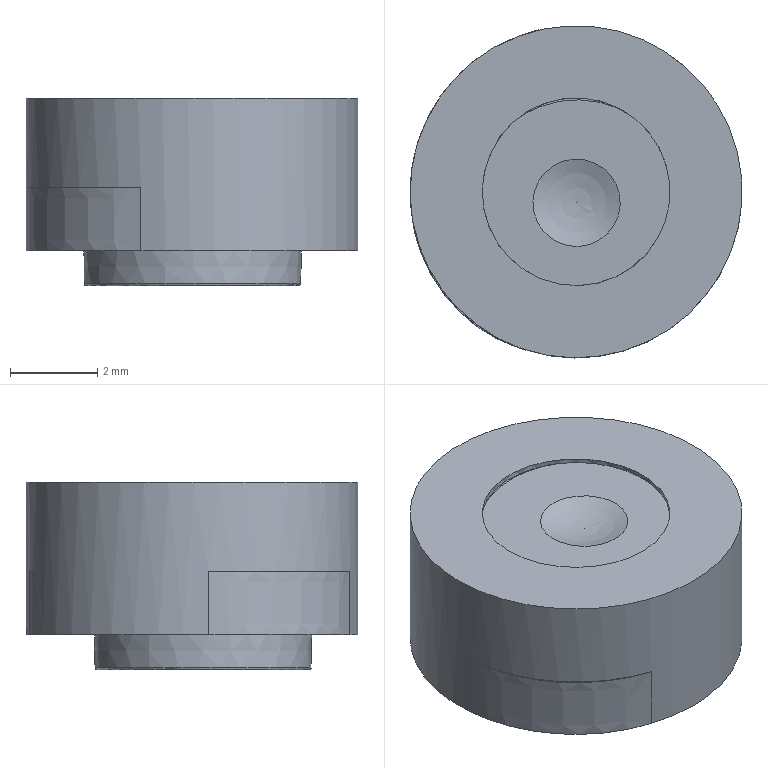Part | STEP file | 1 solid | 29 faces | box 7.6 x 7.6 x 4.3 mm | volume 142.649 mm3 | plane 14 | cylinder 9 | torus 2 | sphere 2 | other 1 | cone 1 | commonest cylinder face diameters 0.1 x6 4.3 x1 7.6 x1 8.471 x1
STEP:
#1=CARTESIAN_POINT('',(24.063,11.212,-13.81));
#2=VERTEX_POINT('',#1);
#3=CARTESIAN_POINT('',(21.454,14.437,-13.81));
#4=VERTEX_POINT('',#3);
#5=CARTESIAN_POINT('',(25.234,14.827,-13.81));
#6=DIRECTION('',(0.,0.,-1.));
#7=DIRECTION('',(-0.3082,-0.9513,0.));
#8=AXIS2_PLACEMENT_3D('',#5,#6,#7);
#9=CIRCLE('',#8,3.8);
#10=EDGE_CURVE('',#2,#4,#9,.T.);
#11=ORIENTED_EDGE('',*,*,#10,.T.);
#12=CARTESIAN_POINT('',(21.454,14.437,-13.81));
#13=CARTESIAN_POINT('',(21.456,14.416,-13.81));
#14=CARTESIAN_POINT('',(21.46,14.376,-13.81));
#15=CARTESIAN_POINT('',(21.467,14.316,-13.81));
#16=CARTESIAN_POINT('',(21.474,14.255,-13.81));
#17=CARTESIAN_POINT('',(21.48,14.215,-13.81));
#18=CARTESIAN_POINT('',(21.486,14.175,-13.81));
#19=CARTESIAN_POINT('',(21.493,14.135,-13.81));
#20=CARTESIAN_POINT('',(21.503,14.076,-13.81));
#21=CARTESIAN_POINT('',(21.515,14.017,-13.81));
#22=CARTESIAN_POINT('',(21.527,13.958,-13.81));
#23=CARTESIAN_POINT('',(21.54,13.899,-13.81));
#24=CARTESIAN_POINT('',(21.554,13.841,-13.81));
#25=CARTESIAN_POINT('',(21.569,13.783,-13.81));
#26=CARTESIAN_POINT('',(21.58,13.745,-13.81));
#27=CARTESIAN_POINT('',(21.591,13.706,-13.81));
#28=CARTESIAN_POINT('',(21.603,13.667,-13.81));
#29=CARTESIAN_POINT('',(21.62,13.61,-13.81));
#30=CARTESIAN_POINT('',(21.639,13.554,-13.81));
#31=CARTESIAN_POINT('',(21.659,13.498,-13.81));
#32=CARTESIAN_POINT('',(21.679,13.441,-13.81));
#33=CARTESIAN_POINT('',(21.701,13.384,-13.81));
#34=CARTESIAN_POINT('',(21.723,13.331,-13.81));
#35=CARTESIAN_POINT('',(21.74,13.291,-13.81));
#36=CARTESIAN_POINT('',(21.758,13.248,-13.81));
#37=CARTESIAN_POINT('',(21.782,13.194,-13.81));
#38=CARTESIAN_POINT('',(21.816,13.123,-13.81));
#39=CARTESIAN_POINT('',(21.842,13.07,-13.81));
#40=CARTESIAN_POINT('',(21.878,13.001,-13.81));
#41=CARTESIAN_POINT('',(21.919,12.925,-13.81));
#42=CARTESIAN_POINT('',(21.966,12.844,-13.81));
#43=CARTESIAN_POINT('',(22.015,12.764,-13.81));
#44=CARTESIAN_POINT('',(22.065,12.686,-13.81));
#45=CARTESIAN_POINT('',(22.127,12.597,-13.81));
#46=CARTESIAN_POINT('',(22.179,12.526,-13.81));
#47=CARTESIAN_POINT('',(22.217,12.476,-13.81));
#48=CARTESIAN_POINT('',(22.249,12.434,-13.81));
#49=CARTESIAN_POINT('',(22.285,12.391,-13.81));
#50=CARTESIAN_POINT('',(22.337,12.328,-13.81));
#51=CARTESIAN_POINT('',(22.409,12.247,-13.81));
#52=CARTESIAN_POINT('',(22.48,12.171,-13.81));
#53=CARTESIAN_POINT('',(22.546,12.105,-13.81));
#54=CARTESIAN_POINT('',(22.613,12.041,-13.81));
#55=CARTESIAN_POINT('',(22.686,11.974,-13.81));
#56=CARTESIAN_POINT('',(22.765,11.906,-13.81));
#57=CARTESIAN_POINT('',(22.828,11.854,-13.81));
#58=CARTESIAN_POINT('',(22.871,11.821,-13.81));
#59=CARTESIAN_POINT('',(22.907,11.794,-13.81));
#60=CARTESIAN_POINT('',(22.942,11.767,-13.81));
#61=CARTESIAN_POINT('',(22.991,11.732,-13.81));
#62=CARTESIAN_POINT('',(23.041,11.697,-13.81));
#63=CARTESIAN_POINT('',(23.091,11.663,-13.81));
#64=CARTESIAN_POINT('',(23.142,11.63,-13.81));
#65=CARTESIAN_POINT('',(23.194,11.597,-13.81));
#66=CARTESIAN_POINT('',(23.235,11.573,-13.81));
#67=CARTESIAN_POINT('',(23.271,11.552,-13.81));
#68=CARTESIAN_POINT('',(23.308,11.531,-13.81));
#69=CARTESIAN_POINT('',(23.361,11.501,-13.81));
#70=CARTESIAN_POINT('',(23.426,11.466,-13.81));
#71=CARTESIAN_POINT('',(23.509,11.425,-13.81));
#72=CARTESIAN_POINT('',(23.579,11.392,-13.81));
#73=CARTESIAN_POINT('',(23.654,11.359,-13.81));
#74=CARTESIAN_POINT('',(23.73,11.327,-13.81));
#75=CARTESIAN_POINT('',(23.832,11.288,-13.81));
#76=CARTESIAN_POINT('',(23.906,11.262,-13.81));
#77=CARTESIAN_POINT('',(23.981,11.237,-13.81));
#78=CARTESIAN_POINT('',(24.022,11.224,-13.81));
#79=CARTESIAN_POINT('',(24.063,11.212,-13.81));
#80=B_SPLINE_CURVE_WITH_KNOTS('',3,(#12,#13,#14,#15,#16,#17,#18,#19,#20,#21,#22,#23,#24,#25,#26,#27,#28,#29,#30,#31,#32,#33,#34,#35,#36,#37,#38,#39,#40,#41,#42,#43,#44,#45,#46,#47,#48,#49,#50,#51,#52,#53,#54,#55,#56,#57,#58,#59,#60,#61,#62,#63,#64,#65,#66,#67,#68,#69,#70,#71,#72,#73,#74,#75,#76,#77,#78,#79),.UNSPECIFIED.,.F.,.F.,(4,1,1,1,1,1,1,1,1,1,1,1,1,1,1,1,1,1,1,1,1,1,1,1,1,1,1,1,1,1,1,1,1,1,1,1,1,1,1,1,1,1,1,1,1,1,1,1,1,1,1,1,1,1,1,1,1,1,1,1,1,1,1,1,1,4),(0.,0.01381,0.02762,0.04141,0.05518,0.05537,0.06892,0.08262,0.0963,0.1099,0.1236,0.1372,0.1509,0.164,0.1645,0.1781,0.1916,0.2052,0.2187,0.2321,0.2461,0.2606,0.2707,0.276,0.292,0.311,0.3293,0.3324,0.3643,0.3876,0.3963,0.4283,0.4504,0.4704,0.4885,0.4928,0.5065,0.5266,0.5485,0.5803,0.5972,0.612,0.6435,0.6646,0.6832,0.6989,0.7013,0.7141,0.7285,0.7425,0.756,0.7697,0.7836,0.7978,0.8019,0.8123,0.8269,0.8435,0.8621,0.8898,0.8961,0.9178,0.946,0.971,0.9711,1.),.UNSPECIFIED.);
#81=EDGE_CURVE('',#4,#2,#80,.T.);
#82=ORIENTED_EDGE('',*,*,#81,.T.);
#83=EDGE_LOOP('',(#11,#82));
#84=FACE_BOUND('',#83,.T.);
#85=CARTESIAN_POINT('',(25.245,14.575,-13.81));
#86=DIRECTION('',(0.,0.,1.));
#87=DIRECTION('',(1.,0.,0.));
#88=AXIS2_PLACEMENT_3D('',#85,#86,#87);
#89=PLANE('',#88);
#90=ADVANCED_FACE('',(#84),#89,.T.);
#91=ORIENTED_EDGE('',*,*,#81,.F.);
#92=CARTESIAN_POINT('',(21.454,14.437,-15.26));
#93=VERTEX_POINT('',#92);
#94=CARTESIAN_POINT('',(21.454,14.437,-13.81));
#95=DIRECTION('',(0.,0.,-1.));
#96=VECTOR('',#95,1.);
#97=LINE('',#94,#96);
#98=EDGE_CURVE('',#4,#93,#97,.T.);
#99=ORIENTED_EDGE('',*,*,#98,.T.);
#100=CARTESIAN_POINT('',(24.063,11.212,-15.26));
#101=VERTEX_POINT('',#100);
#102=CARTESIAN_POINT('',(24.063,11.212,-15.26));
#103=CARTESIAN_POINT('',(24.014,11.226,-15.26));
#104=CARTESIAN_POINT('',(23.942,11.249,-15.26));
#105=CARTESIAN_POINT('',(23.846,11.283,-15.26));
#106=CARTESIAN_POINT('',(23.752,11.318,-15.26));
#107=CARTESIAN_POINT('',(23.635,11.366,-15.26));
#108=CARTESIAN_POINT('',(23.52,11.419,-15.26));
#109=CARTESIAN_POINT('',(23.43,11.465,-15.26));
#110=CARTESIAN_POINT('',(23.34,11.512,-15.26));
#111=CARTESIAN_POINT('',(23.229,11.576,-15.26));
#112=CARTESIAN_POINT('',(23.123,11.642,-15.26));
#113=CARTESIAN_POINT('',(23.038,11.699,-15.26));
#114=CARTESIAN_POINT('',(22.955,11.757,-15.26));
#115=CARTESIAN_POINT('',(22.889,11.807,-15.26));
#116=CARTESIAN_POINT('',(22.809,11.87,-15.26));
#117=CARTESIAN_POINT('',(22.742,11.925,-15.26));
#118=CARTESIAN_POINT('',(22.67,11.988,-15.26));
#119=CARTESIAN_POINT('',(22.6,12.052,-15.26));
#120=CARTESIAN_POINT('',(22.526,12.124,-15.26));
#121=CARTESIAN_POINT('',(22.434,12.219,-15.26));
#122=CARTESIAN_POINT('',(22.37,12.29,-15.26));
#123=CARTESIAN_POINT('',(22.316,12.353,-15.26));
#124=CARTESIAN_POINT('',(22.265,12.414,-15.26));
#125=CARTESIAN_POINT('',(22.196,12.502,-15.26));
#126=CARTESIAN_POINT('',(22.125,12.6,-15.26));
#127=CARTESIAN_POINT('',(22.078,12.668,-15.26));
#128=CARTESIAN_POINT('',(22.027,12.745,-15.26));
#129=CARTESIAN_POINT('',(21.964,12.846,-15.26));
#130=CARTESIAN_POINT('',(21.888,12.98,-15.26));
#131=CARTESIAN_POINT('',(21.824,13.105,-15.26));
#132=CARTESIAN_POINT('',(21.765,13.231,-15.26));
#133=CARTESIAN_POINT('',(21.706,13.369,-15.26));
#134=CARTESIAN_POINT('',(21.663,13.484,-15.26));
#135=CARTESIAN_POINT('',(21.634,13.568,-15.26));
#136=CARTESIAN_POINT('',(21.61,13.642,-15.26));
#137=CARTESIAN_POINT('',(21.579,13.745,-15.26));
#138=CARTESIAN_POINT('',(21.553,13.846,-15.26));
#139=CARTESIAN_POINT('',(21.534,13.928,-15.26));
#140=CARTESIAN_POINT('',(21.52,13.99,-15.26));
#141=CARTESIAN_POINT('',(21.508,14.049,-15.26));
#142=CARTESIAN_POINT('',(21.495,14.121,-15.26));
#143=CARTESIAN_POINT('',(21.482,14.204,-15.26));
#144=CARTESIAN_POINT('',(21.472,14.273,-15.26));
#145=CARTESIAN_POINT('',(21.466,14.325,-15.26));
#146=CARTESIAN_POINT('',(21.46,14.376,-15.26));
#147=CARTESIAN_POINT('',(21.457,14.412,-15.26));
#148=CARTESIAN_POINT('',(21.454,14.437,-15.26));
#149=B_SPLINE_CURVE_WITH_KNOTS('',3,(#102,#103,#104,#105,#106,#107,#108,#109,#110,#111,#112,#113,#114,#115,#116,#117,#118,#119,#120,#121,#122,#123,#124,#125,#126,#127,#128,#129,#130,#131,#132,#133,#134,#135,#136,#137,#138,#139,#140,#141,#142,#143,#144,#145,#146,#147,#148),.UNSPECIFIED.,.F.,.F.,(4,1,1,1,1,1,1,1,1,1,1,1,1,1,1,1,1,1,1,1,1,1,1,1,1,1,1,1,1,1,1,1,1,1,1,1,1,1,1,1,1,1,1,1,4),(0.,0.03441,0.05187,0.06883,0.1032,0.1378,0.1548,0.1723,0.207,0.2417,0.257,0.2766,0.3114,0.3132,0.3454,0.3704,0.3786,0.4099,0.4404,0.469,0.4746,0.4968,0.5236,0.5503,0.5794,0.5801,0.6129,0.6604,0.6852,0.708,0.7555,0.7875,0.7914,0.8161,0.8405,0.8644,0.8868,0.8977,0.9081,0.9279,0.9471,0.9653,0.9755,0.9829,1.),.UNSPECIFIED.);
#150=EDGE_CURVE('',#101,#93,#149,.T.);
#151=ORIENTED_EDGE('',*,*,#150,.F.);
#152=CARTESIAN_POINT('',(24.063,11.212,-15.26));
#153=DIRECTION('',(0.,0.,1.));
#154=VECTOR('',#153,1.);
#155=LINE('',#152,#154);
#156=EDGE_CURVE('',#101,#2,#155,.T.);
#157=ORIENTED_EDGE('',*,*,#156,.T.);
#158=EDGE_LOOP('',(#91,#99,#151,#157));
#159=FACE_BOUND('',#158,.T.);
#160=CARTESIAN_POINT('',(24.179,11.181,-13.781));
#161=CARTESIAN_POINT('',(24.14,11.19,-13.781));
#162=CARTESIAN_POINT('',(23.887,11.26,-13.781));
#163=CARTESIAN_POINT('',(23.197,11.533,-13.781));
#164=CARTESIAN_POINT('',(22.25,12.283,-13.781));
#165=CARTESIAN_POINT('',(21.632,13.394,-13.781));
#166=CARTESIAN_POINT('',(21.471,14.194,-13.781));
#167=CARTESIAN_POINT('',(21.448,14.516,-13.781));
#168=CARTESIAN_POINT('',(21.446,14.556,-13.781));
#169=B_SPLINE_CURVE_WITH_KNOTS('',3,(#160,#161,#162,#163,#164,#165,#166,#167,#168),.UNSPECIFIED.,.F.,.F.,(4,1,1,1,1,1,4),(0.,0.02582,0.1691,0.477,0.7911,0.9742,1.),.UNSPECIFIED.);
#170=DIRECTION('',(0.,0.,-1.));
#171=VECTOR('',#170,1.);
#172=SURFACE_OF_LINEAR_EXTRUSION('',#169,#171);
#173=ADVANCED_FACE('',(#159),#172,.T.);
#174=CARTESIAN_POINT('',(28.525,12.927,-11.76));
#175=VERTEX_POINT('',#174);
#176=CARTESIAN_POINT('',(25.234,14.827,-11.76));
#177=DIRECTION('',(0.,0.,1.));
#178=DIRECTION('',(-0.866,0.5,0.));
#179=AXIS2_PLACEMENT_3D('',#176,#177,#178);
#180=CIRCLE('',#179,3.8);
#181=EDGE_CURVE('',#175,#175,#180,.T.);
#182=ORIENTED_EDGE('',*,*,#181,.F.);
#183=EDGE_LOOP('',(#182));
#184=FACE_OUTER_BOUND('',#183,.T.);
#185=CARTESIAN_POINT('',(24.39,18.532,-15.26));
#186=VERTEX_POINT('',#185);
#187=CARTESIAN_POINT('',(28.525,12.927,-15.26));
#188=VERTEX_POINT('',#187);
#189=CARTESIAN_POINT('',(25.234,14.827,-15.26));
#190=DIRECTION('',(0.,0.,-1.));
#191=DIRECTION('',(-0.2221,0.975,0.));
#192=AXIS2_PLACEMENT_3D('',#189,#190,#191);
#193=CIRCLE('',#192,3.8);
#194=EDGE_CURVE('',#186,#188,#193,.T.);
#195=ORIENTED_EDGE('',*,*,#194,.F.);
#196=CARTESIAN_POINT('',(24.39,18.532,-13.81));
#197=VERTEX_POINT('',#196);
#198=CARTESIAN_POINT('',(24.39,18.532,-15.26));
#199=DIRECTION('',(0.,0.,1.));
#200=VECTOR('',#199,1.);
#201=LINE('',#198,#200);
#202=EDGE_CURVE('',#186,#197,#201,.T.);
#203=ORIENTED_EDGE('',*,*,#202,.T.);
#204=CARTESIAN_POINT('',(24.092,18.451,-13.81));
#205=VERTEX_POINT('',#204);
#206=CARTESIAN_POINT('',(25.234,14.827,-13.81));
#207=DIRECTION('',(0.,0.,-1.));
#208=DIRECTION('',(-0.3006,0.9537,0.));
#209=AXIS2_PLACEMENT_3D('',#206,#207,#208);
#210=CIRCLE('',#209,3.8);
#211=EDGE_CURVE('',#205,#197,#210,.T.);
#212=ORIENTED_EDGE('',*,*,#211,.F.);
#213=CARTESIAN_POINT('',(24.092,18.451,-15.26));
#214=VERTEX_POINT('',#213);
#215=CARTESIAN_POINT('',(24.092,18.451,-15.26));
#216=DIRECTION('',(0.,0.,1.));
#217=VECTOR('',#216,1.);
#218=LINE('',#215,#217);
#219=EDGE_CURVE('',#214,#205,#218,.T.);
#220=ORIENTED_EDGE('',*,*,#219,.F.);
#221=CARTESIAN_POINT('',(25.234,14.827,-15.26));
#222=DIRECTION('',(0.,0.,-1.));
#223=DIRECTION('',(-0.9947,-0.1028,0.));
#224=AXIS2_PLACEMENT_3D('',#221,#222,#223);
#225=CIRCLE('',#224,3.8);
#226=EDGE_CURVE('',#93,#214,#225,.T.);
#227=ORIENTED_EDGE('',*,*,#226,.F.);
#228=ORIENTED_EDGE('',*,*,#98,.F.);
#229=ORIENTED_EDGE('',*,*,#10,.F.);
#230=ORIENTED_EDGE('',*,*,#156,.F.);
#231=CARTESIAN_POINT('',(25.234,14.827,-15.26));
#232=DIRECTION('',(0.,0.,-1.));
#233=DIRECTION('',(0.866,-0.5,0.));
#234=AXIS2_PLACEMENT_3D('',#231,#232,#233);
#235=CIRCLE('',#234,3.8);
#236=EDGE_CURVE('',#188,#101,#235,.T.);
#237=ORIENTED_EDGE('',*,*,#236,.F.);
#238=EDGE_LOOP('',(#195,#203,#212,#220,#227,#228,#229,#230,#237));
#239=FACE_BOUND('',#238,.T.);
#240=CARTESIAN_POINT('',(25.234,14.827,-15.26));
#241=DIRECTION('',(0.,0.,1.));
#242=DIRECTION('',(0.866,-0.5,0.));
#243=AXIS2_PLACEMENT_3D('',#240,#241,#242);
#244=CYLINDRICAL_SURFACE('',#243,3.8);
#245=ADVANCED_FACE('',(#184,#239),#244,.T.);
#246=ORIENTED_EDGE('',*,*,#194,.T.);
#247=ORIENTED_EDGE('',*,*,#236,.T.);
#248=ORIENTED_EDGE('',*,*,#150,.T.);
#249=ORIENTED_EDGE('',*,*,#226,.T.);
#250=CARTESIAN_POINT('',(24.375,18.541,-15.26));
#251=VERTEX_POINT('',#250);
#252=CARTESIAN_POINT('',(25.507,14.459,-15.26));
#253=DIRECTION('',(0.,0.,-1.));
#254=DIRECTION('',(-0.3341,0.9425,0.));
#255=AXIS2_PLACEMENT_3D('',#252,#253,#254);
#256=CIRCLE('',#255,4.236);
#257=EDGE_CURVE('',#214,#251,#256,.T.);
#258=ORIENTED_EDGE('',*,*,#257,.T.);
#259=CARTESIAN_POINT('',(24.375,18.541,-15.26));
#260=DIRECTION('',(0.866,-0.5,0.));
#261=VECTOR('',#260,1.);
#262=LINE('',#259,#261);
#263=EDGE_CURVE('',#251,#186,#262,.T.);
#264=ORIENTED_EDGE('',*,*,#263,.T.);
#265=EDGE_LOOP('',(#246,#247,#248,#249,#258,#264));
#266=FACE_BOUND('',#265,.T.);
#267=CARTESIAN_POINT('',(23.088,15.82,-15.26));
#268=VERTEX_POINT('',#267);
#269=CARTESIAN_POINT('',(25.245,14.575,-15.26));
#270=DIRECTION('',(0.,0.,1.));
#271=DIRECTION('',(1.,0.,0.));
#272=AXIS2_PLACEMENT_3D('',#269,#270,#271);
#273=CIRCLE('',#272,2.49);
#274=EDGE_CURVE('',#268,#268,#273,.T.);
#275=ORIENTED_EDGE('',*,*,#274,.T.);
#276=EDGE_LOOP('',(#275));
#277=FACE_BOUND('',#276,.T.);
#278=CARTESIAN_POINT('',(25.245,14.575,-15.26));
#279=DIRECTION('',(0.,0.,1.));
#280=DIRECTION('',(1.,0.,0.));
#281=AXIS2_PLACEMENT_3D('',#278,#279,#280);
#282=PLANE('',#281);
#283=ADVANCED_FACE('',(#266,#277),#282,.F.);
#284=CARTESIAN_POINT('',(24.375,18.541,-13.81));
#285=VERTEX_POINT('',#284);
#286=CARTESIAN_POINT('',(24.39,18.532,-13.81));
#287=DIRECTION('',(-0.866,0.5,0.));
#288=VECTOR('',#287,1.);
#289=LINE('',#286,#288);
#290=EDGE_CURVE('',#197,#285,#289,.T.);
#291=ORIENTED_EDGE('',*,*,#290,.F.);
#292=ORIENTED_EDGE('',*,*,#202,.F.);
#293=ORIENTED_EDGE('',*,*,#263,.F.);
#294=CARTESIAN_POINT('',(24.375,18.541,-13.81));
#295=DIRECTION('',(0.,0.,-1.));
#296=VECTOR('',#295,1.);
#297=LINE('',#294,#296);
#298=EDGE_CURVE('',#285,#251,#297,.T.);
#299=ORIENTED_EDGE('',*,*,#298,.F.);
#300=EDGE_LOOP('',(#291,#292,#293,#299));
#301=FACE_BOUND('',#300,.T.);
#302=CARTESIAN_POINT('',(26.745,17.173,-15.26));
#303=DIRECTION('',(-0.5,-0.866,0.));
#304=DIRECTION('',(-0.866,0.5,0.));
#305=AXIS2_PLACEMENT_3D('',#302,#303,#304);
#306=PLANE('',#305);
#307=ADVANCED_FACE('',(#301),#306,.F.);
#308=CARTESIAN_POINT('',(25.507,14.459,-13.81));
#309=DIRECTION('',(0.,0.,1.));
#310=DIRECTION('',(-0.2671,0.9637,0.));
#311=AXIS2_PLACEMENT_3D('',#308,#309,#310);
#312=CIRCLE('',#311,4.236);
#313=EDGE_CURVE('',#285,#205,#312,.T.);
#314=ORIENTED_EDGE('',*,*,#313,.F.);
#315=ORIENTED_EDGE('',*,*,#298,.T.);
#316=ORIENTED_EDGE('',*,*,#257,.F.);
#317=ORIENTED_EDGE('',*,*,#219,.T.);
#318=EDGE_LOOP('',(#314,#315,#316,#317));
#319=FACE_BOUND('',#318,.T.);
#320=CARTESIAN_POINT('',(25.507,14.459,-14.535));
#321=DIRECTION('',(0.,0.,1.));
#322=DIRECTION('',(-0.3341,0.9425,0.));
#323=AXIS2_PLACEMENT_3D('',#320,#321,#322);
#324=CYLINDRICAL_SURFACE('',#323,4.236);
#325=ADVANCED_FACE('',(#319),#324,.T.);
#326=ORIENTED_EDGE('',*,*,#313,.T.);
#327=ORIENTED_EDGE('',*,*,#211,.T.);
#328=ORIENTED_EDGE('',*,*,#290,.T.);
#329=EDGE_LOOP('',(#326,#327,#328));
#330=FACE_BOUND('',#329,.T.);
#331=CARTESIAN_POINT('',(25.245,14.575,-13.81));
#332=DIRECTION('',(0.,0.,1.));
#333=DIRECTION('',(1.,0.,0.));
#334=AXIS2_PLACEMENT_3D('',#331,#332,#333);
#335=PLANE('',#334);
#336=ADVANCED_FACE('',(#330),#335,.T.);
#337=CARTESIAN_POINT('',(23.1,15.813,-16.011));
#338=VERTEX_POINT('',#337);
#339=CARTESIAN_POINT('',(23.1,15.813,-16.011));
#340=CARTESIAN_POINT('',(23.126,15.858,-16.011));
#341=CARTESIAN_POINT('',(23.18,15.947,-16.011));
#342=CARTESIAN_POINT('',(23.27,16.074,-16.011));
#343=CARTESIAN_POINT('',(23.368,16.195,-16.011));
#344=CARTESIAN_POINT('',(23.474,16.309,-16.011));
#345=CARTESIAN_POINT('',(23.586,16.417,-16.011));
#346=CARTESIAN_POINT('',(23.705,16.517,-16.011));
#347=CARTESIAN_POINT('',(23.83,16.61,-16.011));
#348=CARTESIAN_POINT('',(23.961,16.695,-16.011));
#349=CARTESIAN_POINT('',(24.097,16.772,-16.011));
#350=CARTESIAN_POINT('',(24.237,16.839,-16.011));
#351=CARTESIAN_POINT('',(24.381,16.898,-16.011));
#352=CARTESIAN_POINT('',(24.529,16.948,-16.011));
#353=CARTESIAN_POINT('',(24.679,16.988,-16.011));
#354=CARTESIAN_POINT('',(24.832,17.019,-16.011));
#355=CARTESIAN_POINT('',(24.986,17.04,-16.011));
#356=CARTESIAN_POINT('',(25.141,17.051,-16.011));
#357=CARTESIAN_POINT('',(25.297,17.053,-16.011));
#358=CARTESIAN_POINT('',(25.452,17.045,-16.011));
#359=CARTESIAN_POINT('',(25.607,17.027,-16.011));
#360=CARTESIAN_POINT('',(25.76,16.999,-16.011));
#361=CARTESIAN_POINT('',(25.912,16.962,-16.011));
#362=CARTESIAN_POINT('',(26.06,16.915,-16.011));
#363=CARTESIAN_POINT('',(26.206,16.86,-16.011));
#364=CARTESIAN_POINT('',(26.347,16.795,-16.011));
#365=CARTESIAN_POINT('',(26.484,16.721,-16.011));
#366=CARTESIAN_POINT('',(26.617,16.639,-16.011));
#367=CARTESIAN_POINT('',(26.744,16.549,-16.011));
#368=CARTESIAN_POINT('',(26.865,16.451,-16.011));
#369=CARTESIAN_POINT('',(26.979,16.345,-16.011));
#370=CARTESIAN_POINT('',(27.087,16.233,-16.011));
#371=CARTESIAN_POINT('',(27.188,16.114,-16.011));
#372=CARTESIAN_POINT('',(27.28,15.989,-16.011));
#373=CARTESIAN_POINT('',(27.365,15.858,-16.011));
#374=CARTESIAN_POINT('',(27.442,15.723,-16.011));
#375=CARTESIAN_POINT('',(27.509,15.582,-16.011));
#376=CARTESIAN_POINT('',(27.568,15.438,-16.011));
#377=CARTESIAN_POINT('',(27.618,15.29,-16.011));
#378=CARTESIAN_POINT('',(27.658,15.14,-16.011));
#379=CARTESIAN_POINT('',(27.689,14.987,-16.011));
#380=CARTESIAN_POINT('',(27.71,14.833,-16.011));
#381=CARTESIAN_POINT('',(27.721,14.678,-16.011));
#382=CARTESIAN_POINT('',(27.723,14.522,-16.011));
#383=CARTESIAN_POINT('',(27.714,14.367,-16.011));
#384=CARTESIAN_POINT('',(27.696,14.212,-16.011));
#385=CARTESIAN_POINT('',(27.669,14.059,-16.011));
#386=CARTESIAN_POINT('',(27.632,13.907,-16.011));
#387=CARTESIAN_POINT('',(27.585,13.759,-16.011));
#388=CARTESIAN_POINT('',(27.529,13.613,-16.011));
#389=CARTESIAN_POINT('',(27.464,13.472,-16.011));
#390=CARTESIAN_POINT('',(27.415,13.381,-16.011));
#391=CARTESIAN_POINT('',(27.39,13.337,-16.011));
#392=CARTESIAN_POINT('',(27.364,13.292,-16.011));
#393=CARTESIAN_POINT('',(27.309,13.203,-16.011));
#394=CARTESIAN_POINT('',(27.219,13.076,-16.011));
#395=CARTESIAN_POINT('',(27.121,12.955,-16.011));
#396=CARTESIAN_POINT('',(27.015,12.841,-16.011));
#397=CARTESIAN_POINT('',(26.903,12.733,-16.011));
#398=CARTESIAN_POINT('',(26.784,12.633,-16.011));
#399=CARTESIAN_POINT('',(26.659,12.54,-16.011));
#400=CARTESIAN_POINT('',(26.528,12.455,-16.011));
#401=CARTESIAN_POINT('',(26.393,12.378,-16.011));
#402=CARTESIAN_POINT('',(26.253,12.311,-16.011));
#403=CARTESIAN_POINT('',(26.108,12.252,-16.011));
#404=CARTESIAN_POINT('',(25.961,12.202,-16.011));
#405=CARTESIAN_POINT('',(25.81,12.162,-16.011));
#406=CARTESIAN_POINT('',(25.658,12.131,-16.011));
#407=CARTESIAN_POINT('',(25.503,12.11,-16.011));
#408=CARTESIAN_POINT('',(25.348,12.099,-16.011));
#409=CARTESIAN_POINT('',(25.192,12.097,-16.011));
#410=CARTESIAN_POINT('',(25.037,12.105,-16.011));
#411=CARTESIAN_POINT('',(24.882,12.123,-16.011));
#412=CARTESIAN_POINT('',(24.729,12.151,-16.011));
#413=CARTESIAN_POINT('',(24.578,12.188,-16.011));
#414=CARTESIAN_POINT('',(24.429,12.235,-16.011));
#415=CARTESIAN_POINT('',(24.284,12.29,-16.011));
#416=CARTESIAN_POINT('',(24.142,12.355,-16.011));
#417=CARTESIAN_POINT('',(24.005,12.429,-16.011));
#418=CARTESIAN_POINT('',(23.873,12.511,-16.011));
#419=CARTESIAN_POINT('',(23.746,12.601,-16.011));
#420=CARTESIAN_POINT('',(23.625,12.699,-16.011));
#421=CARTESIAN_POINT('',(23.51,12.805,-16.011));
#422=CARTESIAN_POINT('',(23.402,12.917,-16.011));
#423=CARTESIAN_POINT('',(23.302,13.036,-16.011));
#424=CARTESIAN_POINT('',(23.209,13.161,-16.011));
#425=CARTESIAN_POINT('',(23.124,13.292,-16.011));
#426=CARTESIAN_POINT('',(23.048,13.427,-16.011));
#427=CARTESIAN_POINT('',(22.98,13.568,-16.011));
#428=CARTESIAN_POINT('',(22.921,13.712,-16.011));
#429=CARTESIAN_POINT('',(22.872,13.86,-16.011));
#430=CARTESIAN_POINT('',(22.831,14.01,-16.011));
#431=CARTESIAN_POINT('',(22.801,14.163,-16.011));
#432=CARTESIAN_POINT('',(22.78,14.317,-16.011));
#433=CARTESIAN_POINT('',(22.768,14.472,-16.011));
#434=CARTESIAN_POINT('',(22.767,14.628,-16.011));
#435=CARTESIAN_POINT('',(22.775,14.783,-16.011));
#436=CARTESIAN_POINT('',(22.793,14.938,-16.011));
#437=CARTESIAN_POINT('',(22.821,15.091,-16.011));
#438=CARTESIAN_POINT('',(22.858,15.243,-16.011));
#439=CARTESIAN_POINT('',(22.904,15.391,-16.011));
#440=CARTESIAN_POINT('',(22.96,15.537,-16.011));
#441=CARTESIAN_POINT('',(23.025,15.678,-16.011));
#442=CARTESIAN_POINT('',(23.074,15.769,-16.011));
#443=CARTESIAN_POINT('',(23.1,15.813,-16.011));
#444=B_SPLINE_CURVE_WITH_KNOTS('',3,(#339,#340,#341,#342,#343,#344,#345,#346,#347,#348,#349,#350,#351,#352,#353,#354,#355,#356,#357,#358,#359,#360,#361,#362,#363,#364,#365,#366,#367,#368,#369,#370,#371,#372,#373,#374,#375,#376,#377,#378,#379,#380,#381,#382,#383,#384,#385,#386,#387,#388,#389,#390,#391,#392,#393,#394,#395,#396,#397,#398,#399,#400,#401,#402,#403,#404,#405,#406,#407,#408,#409,#410,#411,#412,#413,#414,#415,#416,#417,#418,#419,#420,#421,#422,#423,#424,#425,#426,#427,#428,#429,#430,#431,#432,#433,#434,#435,#436,#437,#438,#439,#440,#441,#442,#443),.UNSPECIFIED.,.T.,.F.,(4,1,1,1,1,1,1,1,1,1,1,1,1,1,1,1,1,1,1,1,1,1,1,1,1,1,1,1,1,1,1,1,1,1,1,1,1,1,1,1,1,1,1,1,1,1,1,1,1,1,3,1,1,1,1,1,1,1,1,1,1,1,1,1,1,1,1,1,1,1,1,1,1,1,1,1,1,1,1,1,1,1,1,1,1,1,1,1,1,1,1,1,1,1,1,1,1,1,1,1,4),(0.,0.01,0.02,0.03,0.04001,0.05001,0.06001,0.07001,0.08001,0.09001,0.1,0.11,0.12,0.13,0.14,0.15,0.16,0.17,0.18,0.19,0.2,0.21,0.22,0.23,0.24,0.25,0.26,0.27,0.28,0.29,0.3,0.31,0.3201,0.3301,0.3401,0.3501,0.3601,0.3701,0.3801,0.3901,0.4001,0.4101,0.4201,0.4301,0.4401,0.4501,0.4601,0.4701,0.4801,0.4901,0.5,0.51,0.52,0.53,0.54,0.55,0.56,0.57,0.58,0.59,0.6,0.61,0.62,0.63,0.64,0.65,0.66,0.67,0.68,0.69,0.7,0.71,0.72,0.73,0.74,0.75,0.76,0.77,0.78,0.79,0.8,0.81,0.8201,0.8301,0.8401,0.8501,0.8601,0.8701,0.8801,0.8901,0.9001,0.9101,0.9201,0.9301,0.9401,0.9501,0.9601,0.9701,0.9801,0.9901,1.),.UNSPECIFIED.);
#445=EDGE_CURVE('',#338,#338,#444,.T.);
#446=ORIENTED_EDGE('',*,*,#445,.F.);
#447=EDGE_LOOP('',(#446));
#448=FACE_OUTER_BOUND('',#447,.T.);
#449=ORIENTED_EDGE('',*,*,#274,.F.);
#450=EDGE_LOOP('',(#449));
#451=FACE_OUTER_BOUND('',#450,.T.);
#452=CARTESIAN_POINT('',(25.245,14.575,-15.635));
#453=DIRECTION('',(0.,0.,1.));
#454=DIRECTION('',(0.866,-0.5,0.));
#455=AXIS2_PLACEMENT_3D('',#452,#453,#454);
#456=CONICAL_SURFACE('',#455,2.483,0.01745);
#457=ADVANCED_FACE('',(#448,#451),#456,.T.);
#458=CARTESIAN_POINT('',(23.143,15.788,-16.06));
#459=VERTEX_POINT('',#458);
#460=CARTESIAN_POINT('',(25.245,14.575,-16.06));
#461=DIRECTION('',(0.,0.,-1.));
#462=DIRECTION('',(0.866,-0.5,0.));
#463=AXIS2_PLACEMENT_3D('',#460,#461,#462);
#464=CIRCLE('',#463,2.427);
#465=EDGE_CURVE('',#459,#459,#464,.T.);
#466=ORIENTED_EDGE('',*,*,#465,.F.);
#467=EDGE_LOOP('',(#466));
#468=FACE_OUTER_BOUND('',#467,.T.);
#469=ORIENTED_EDGE('',*,*,#445,.T.);
#470=EDGE_LOOP('',(#469));
#471=FACE_OUTER_BOUND('',#470,.T.);
#472=CARTESIAN_POINT('',(25.245,14.575,-16.01));
#473=DIRECTION('',(0.,0.,1.));
#474=DIRECTION('',(0.866,-0.5,0.));
#475=AXIS2_PLACEMENT_3D('',#472,#473,#474);
#476=TOROIDAL_SURFACE('',#475,2.427,0.05);
#477=ADVANCED_FACE('',(#468,#471),#476,.T.);
#478=ORIENTED_EDGE('',*,*,#465,.T.);
#479=EDGE_LOOP('',(#478));
#480=FACE_BOUND('',#479,.T.);
#481=CARTESIAN_POINT('',(26.875,13.634,-16.06));
#482=VERTEX_POINT('',#481);
#483=CARTESIAN_POINT('',(26.875,15.516,-16.06));
#484=VERTEX_POINT('',#483);
#485=CARTESIAN_POINT('',(26.875,13.634,-16.06));
#486=DIRECTION('',(0.,1.,0.));
#487=VECTOR('',#486,1.);
#488=LINE('',#485,#487);
#489=EDGE_CURVE('',#482,#484,#488,.T.);
#490=ORIENTED_EDGE('',*,*,#489,.T.);
#491=CARTESIAN_POINT('',(25.245,16.457,-16.06));
#492=VERTEX_POINT('',#491);
#493=CARTESIAN_POINT('',(25.245,16.457,-16.06));
#494=DIRECTION('',(0.866,-0.5,0.));
#495=VECTOR('',#494,1.);
#496=LINE('',#493,#495);
#497=EDGE_CURVE('',#492,#484,#496,.T.);
#498=ORIENTED_EDGE('',*,*,#497,.F.);
#499=CARTESIAN_POINT('',(23.615,15.516,-16.06));
#500=VERTEX_POINT('',#499);
#501=CARTESIAN_POINT('',(25.245,16.457,-16.06));
#502=DIRECTION('',(-0.866,-0.5,0.));
#503=VECTOR('',#502,1.);
#504=LINE('',#501,#503);
#505=EDGE_CURVE('',#492,#500,#504,.T.);
#506=ORIENTED_EDGE('',*,*,#505,.T.);
#507=CARTESIAN_POINT('',(23.615,13.634,-16.06));
#508=VERTEX_POINT('',#507);
#509=CARTESIAN_POINT('',(23.615,15.516,-16.06));
#510=DIRECTION('',(0.,-1.,0.));
#511=VECTOR('',#510,1.);
#512=LINE('',#509,#511);
#513=EDGE_CURVE('',#500,#508,#512,.T.);
#514=ORIENTED_EDGE('',*,*,#513,.T.);
#515=CARTESIAN_POINT('',(25.245,12.693,-16.06));
#516=VERTEX_POINT('',#515);
#517=CARTESIAN_POINT('',(25.245,12.693,-16.06));
#518=DIRECTION('',(-0.866,0.5,0.));
#519=VECTOR('',#518,1.);
#520=LINE('',#517,#519);
#521=EDGE_CURVE('',#516,#508,#520,.T.);
#522=ORIENTED_EDGE('',*,*,#521,.F.);
#523=CARTESIAN_POINT('',(25.245,12.693,-16.06));
#524=DIRECTION('',(0.866,0.5,0.));
#525=VECTOR('',#524,1.);
#526=LINE('',#523,#525);
#527=EDGE_CURVE('',#516,#482,#526,.T.);
#528=ORIENTED_EDGE('',*,*,#527,.T.);
#529=EDGE_LOOP('',(#490,#498,#506,#514,#522,#528));
#530=FACE_BOUND('',#529,.T.);
#531=CARTESIAN_POINT('',(25.245,14.575,-16.06));
#532=DIRECTION('',(0.,0.,1.));
#533=DIRECTION('',(1.,0.,0.));
#534=AXIS2_PLACEMENT_3D('',#531,#532,#533);
#535=PLANE('',#534);
#536=ADVANCED_FACE('',(#480,#530),#535,.F.);
#537=CARTESIAN_POINT('',(25.245,12.751,-16.01));
#538=VERTEX_POINT('',#537);
#539=CARTESIAN_POINT('',(26.825,13.663,-16.01));
#540=VERTEX_POINT('',#539);
#541=CARTESIAN_POINT('',(25.245,12.751,-16.01));
#542=DIRECTION('',(0.866,0.5,0.));
#543=VECTOR('',#542,1.);
#544=LINE('',#541,#543);
#545=EDGE_CURVE('',#538,#540,#544,.T.);
#546=ORIENTED_EDGE('',*,*,#545,.T.);
#547=CARTESIAN_POINT('',(26.825,13.663,-16.01));
#548=CARTESIAN_POINT('',(26.825,13.663,-16.039));
#549=CARTESIAN_POINT('',(26.845,13.651,-16.06));
#550=CARTESIAN_POINT('',(26.875,13.634,-16.06));
#551=(BOUNDED_CURVE()B_SPLINE_CURVE(3,(#547,#548,#549,#550),.UNSPECIFIED.,.F.,.F.)B_SPLINE_CURVE_WITH_KNOTS((4,4),(0.,1.),.UNSPECIFIED.)CURVE()GEOMETRIC_REPRESENTATION_ITEM()RATIONAL_B_SPLINE_CURVE((1.,0.8047,0.8047,1.))REPRESENTATION_ITEM(''));
#552=EDGE_CURVE('',#540,#482,#551,.T.);
#553=ORIENTED_EDGE('',*,*,#552,.T.);
#554=ORIENTED_EDGE('',*,*,#527,.F.);
#555=CARTESIAN_POINT('',(25.245,12.751,-16.01));
#556=CARTESIAN_POINT('',(25.245,12.751,-16.039));
#557=CARTESIAN_POINT('',(25.245,12.727,-16.06));
#558=CARTESIAN_POINT('',(25.245,12.693,-16.06));
#559=(BOUNDED_CURVE()B_SPLINE_CURVE(3,(#555,#556,#557,#558),.UNSPECIFIED.,.F.,.F.)B_SPLINE_CURVE_WITH_KNOTS((4,4),(0.,1.),.UNSPECIFIED.)CURVE()GEOMETRIC_REPRESENTATION_ITEM()RATIONAL_B_SPLINE_CURVE((1.,0.8047,0.8047,1.))REPRESENTATION_ITEM(''));
#560=EDGE_CURVE('',#538,#516,#559,.T.);
#561=ORIENTED_EDGE('',*,*,#560,.F.);
#562=EDGE_LOOP('',(#546,#553,#554,#561));
#563=FACE_BOUND('',#562,.T.);
#564=CARTESIAN_POINT('',(24.422,12.218,-16.01));
#565=DIRECTION('',(-0.866,-0.5,0.));
#566=DIRECTION('',(0.,0.,-1.));
#567=AXIS2_PLACEMENT_3D('',#564,#565,#566);
#568=CYLINDRICAL_SURFACE('',#567,0.05);
#569=ADVANCED_FACE('',(#563),#568,.T.);
#570=ORIENTED_EDGE('',*,*,#521,.T.);
#571=CARTESIAN_POINT('',(23.665,13.663,-16.01));
#572=VERTEX_POINT('',#571);
#573=CARTESIAN_POINT('',(23.615,13.634,-16.06));
#574=CARTESIAN_POINT('',(23.644,13.651,-16.06));
#575=CARTESIAN_POINT('',(23.665,13.663,-16.039));
#576=CARTESIAN_POINT('',(23.665,13.663,-16.01));
#577=(BOUNDED_CURVE()B_SPLINE_CURVE(3,(#573,#574,#575,#576),.UNSPECIFIED.,.F.,.F.)B_SPLINE_CURVE_WITH_KNOTS((4,4),(0.,1.),.UNSPECIFIED.)CURVE()GEOMETRIC_REPRESENTATION_ITEM()RATIONAL_B_SPLINE_CURVE((1.,0.8047,0.8047,1.))REPRESENTATION_ITEM(''));
#578=EDGE_CURVE('',#508,#572,#577,.T.);
#579=ORIENTED_EDGE('',*,*,#578,.T.);
#580=CARTESIAN_POINT('',(23.665,13.663,-16.01));
#581=DIRECTION('',(0.866,-0.5,0.));
#582=VECTOR('',#581,1.);
#583=LINE('',#580,#582);
#584=EDGE_CURVE('',#572,#538,#583,.T.);
#585=ORIENTED_EDGE('',*,*,#584,.T.);
#586=ORIENTED_EDGE('',*,*,#560,.T.);
#587=EDGE_LOOP('',(#570,#579,#585,#586));
#588=FACE_BOUND('',#587,.T.);
#589=CARTESIAN_POINT('',(22.305,14.39,-16.01));
#590=DIRECTION('',(-0.866,0.5,0.));
#591=DIRECTION('',(0.,0.,-1.));
#592=AXIS2_PLACEMENT_3D('',#589,#590,#591);
#593=CYLINDRICAL_SURFACE('',#592,0.05);
#594=ADVANCED_FACE('',(#588),#593,.T.);
#595=CARTESIAN_POINT('',(23.665,13.663,-12.56));
#596=VERTEX_POINT('',#595);
#597=CARTESIAN_POINT('',(25.245,12.751,-12.56));
#598=VERTEX_POINT('',#597);
#599=CARTESIAN_POINT('',(23.665,13.663,-12.56));
#600=DIRECTION('',(0.866,-0.5,0.));
#601=VECTOR('',#600,1.);
#602=LINE('',#599,#601);
#603=EDGE_CURVE('',#596,#598,#602,.T.);
#604=ORIENTED_EDGE('',*,*,#603,.T.);
#605=CARTESIAN_POINT('',(25.245,12.751,-12.56));
#606=DIRECTION('',(0.,0.,-1.));
#607=VECTOR('',#606,1.);
#608=LINE('',#605,#607);
#609=EDGE_CURVE('',#598,#538,#608,.T.);
#610=ORIENTED_EDGE('',*,*,#609,.T.);
#611=ORIENTED_EDGE('',*,*,#584,.F.);
#612=CARTESIAN_POINT('',(23.665,13.663,-16.01));
#613=DIRECTION('',(0.,0.,1.));
#614=VECTOR('',#613,1.);
#615=LINE('',#612,#614);
#616=EDGE_CURVE('',#572,#596,#615,.T.);
#617=ORIENTED_EDGE('',*,*,#616,.T.);
#618=EDGE_LOOP('',(#604,#610,#611,#617));
#619=FACE_BOUND('',#618,.T.);
#620=CARTESIAN_POINT('',(25.245,12.751,-16.06));
#621=DIRECTION('',(-0.5,-0.866,0.));
#622=DIRECTION('',(-0.866,0.5,0.));
#623=AXIS2_PLACEMENT_3D('',#620,#621,#622);
#624=PLANE('',#623);
#625=ADVANCED_FACE('',(#619),#624,.F.);
#626=CARTESIAN_POINT('',(23.665,15.487,-12.56));
#627=VERTEX_POINT('',#626);
#628=CARTESIAN_POINT('',(23.665,13.663,-12.56));
#629=DIRECTION('',(0.,1.,0.));
#630=VECTOR('',#629,1.);
#631=LINE('',#628,#630);
#632=EDGE_CURVE('',#596,#627,#631,.T.);
#633=ORIENTED_EDGE('',*,*,#632,.F.);
#634=ORIENTED_EDGE('',*,*,#616,.F.);
#635=CARTESIAN_POINT('',(23.665,15.487,-16.01));
#636=VERTEX_POINT('',#635);
#637=CARTESIAN_POINT('',(23.665,15.487,-16.01));
#638=DIRECTION('',(0.,-1.,0.));
#639=VECTOR('',#638,1.);
#640=LINE('',#637,#639);
#641=EDGE_CURVE('',#636,#572,#640,.T.);
#642=ORIENTED_EDGE('',*,*,#641,.F.);
#643=CARTESIAN_POINT('',(23.665,15.487,-16.01));
#644=DIRECTION('',(0.,0.,1.));
#645=VECTOR('',#644,1.);
#646=LINE('',#643,#645);
#647=EDGE_CURVE('',#636,#627,#646,.T.);
#648=ORIENTED_EDGE('',*,*,#647,.T.);
#649=EDGE_LOOP('',(#633,#634,#642,#648));
#650=FACE_BOUND('',#649,.T.);
#651=CARTESIAN_POINT('',(23.665,13.663,-16.06));
#652=DIRECTION('',(-1.,0.,0.));
#653=DIRECTION('',(0.,1.,0.));
#654=AXIS2_PLACEMENT_3D('',#651,#652,#653);
#655=PLANE('',#654);
#656=ADVANCED_FACE('',(#650),#655,.F.);
#657=CARTESIAN_POINT('',(25.245,16.399,-12.56));
#658=VERTEX_POINT('',#657);
#659=CARTESIAN_POINT('',(23.665,15.487,-12.56));
#660=DIRECTION('',(0.866,0.5,0.));
#661=VECTOR('',#660,1.);
#662=LINE('',#659,#661);
#663=EDGE_CURVE('',#627,#658,#662,.T.);
#664=ORIENTED_EDGE('',*,*,#663,.F.);
#665=ORIENTED_EDGE('',*,*,#647,.F.);
#666=CARTESIAN_POINT('',(25.245,16.399,-16.01));
#667=VERTEX_POINT('',#666);
#668=CARTESIAN_POINT('',(25.245,16.399,-16.01));
#669=DIRECTION('',(-0.866,-0.5,0.));
#670=VECTOR('',#669,1.);
#671=LINE('',#668,#670);
#672=EDGE_CURVE('',#667,#636,#671,.T.);
#673=ORIENTED_EDGE('',*,*,#672,.F.);
#674=CARTESIAN_POINT('',(25.245,16.399,-16.01));
#675=DIRECTION('',(0.,0.,1.));
#676=VECTOR('',#675,1.);
#677=LINE('',#674,#676);
#678=EDGE_CURVE('',#667,#658,#677,.T.);
#679=ORIENTED_EDGE('',*,*,#678,.T.);
#680=EDGE_LOOP('',(#664,#665,#673,#679));
#681=FACE_BOUND('',#680,.T.);
#682=CARTESIAN_POINT('',(23.665,15.487,-16.06));
#683=DIRECTION('',(-0.5,0.866,0.));
#684=DIRECTION('',(0.,0.,1.));
#685=AXIS2_PLACEMENT_3D('',#682,#683,#684);
#686=PLANE('',#685);
#687=ADVANCED_FACE('',(#681),#686,.F.);
#688=CARTESIAN_POINT('',(26.825,15.487,-12.56));
#689=VERTEX_POINT('',#688);
#690=CARTESIAN_POINT('',(25.245,16.399,-12.56));
#691=DIRECTION('',(0.866,-0.5,0.));
#692=VECTOR('',#691,1.);
#693=LINE('',#690,#692);
#694=EDGE_CURVE('',#658,#689,#693,.T.);
#695=ORIENTED_EDGE('',*,*,#694,.F.);
#696=ORIENTED_EDGE('',*,*,#678,.F.);
#697=CARTESIAN_POINT('',(26.825,15.487,-16.01));
#698=VERTEX_POINT('',#697);
#699=CARTESIAN_POINT('',(26.825,15.487,-16.01));
#700=DIRECTION('',(-0.866,0.5,0.));
#701=VECTOR('',#700,1.);
#702=LINE('',#699,#701);
#703=EDGE_CURVE('',#698,#667,#702,.T.);
#704=ORIENTED_EDGE('',*,*,#703,.F.);
#705=CARTESIAN_POINT('',(26.825,15.487,-16.01));
#706=DIRECTION('',(0.,0.,1.));
#707=VECTOR('',#706,1.);
#708=LINE('',#705,#707);
#709=EDGE_CURVE('',#698,#689,#708,.T.);
#710=ORIENTED_EDGE('',*,*,#709,.T.);
#711=EDGE_LOOP('',(#695,#696,#704,#710));
#712=FACE_BOUND('',#711,.T.);
#713=CARTESIAN_POINT('',(25.245,16.399,-16.06));
#714=DIRECTION('',(0.5,0.866,0.));
#715=DIRECTION('',(0.,0.,-1.));
#716=AXIS2_PLACEMENT_3D('',#713,#714,#715);
#717=PLANE('',#716);
#718=ADVANCED_FACE('',(#712),#717,.F.);
#719=CARTESIAN_POINT('',(26.825,13.663,-12.56));
#720=VERTEX_POINT('',#719);
#721=CARTESIAN_POINT('',(26.825,15.487,-12.56));
#722=DIRECTION('',(0.,-1.,0.));
#723=VECTOR('',#722,1.);
#724=LINE('',#721,#723);
#725=EDGE_CURVE('',#689,#720,#724,.T.);
#726=ORIENTED_EDGE('',*,*,#725,.F.);
#727=ORIENTED_EDGE('',*,*,#709,.F.);
#728=CARTESIAN_POINT('',(26.825,13.663,-16.01));
#729=DIRECTION('',(0.,1.,0.));
#730=VECTOR('',#729,1.);
#731=LINE('',#728,#730);
#732=EDGE_CURVE('',#540,#698,#731,.T.);
#733=ORIENTED_EDGE('',*,*,#732,.F.);
#734=CARTESIAN_POINT('',(26.825,13.663,-12.56));
#735=DIRECTION('',(0.,0.,-1.));
#736=VECTOR('',#735,1.);
#737=LINE('',#734,#736);
#738=EDGE_CURVE('',#720,#540,#737,.T.);
#739=ORIENTED_EDGE('',*,*,#738,.F.);
#740=EDGE_LOOP('',(#726,#727,#733,#739));
#741=FACE_BOUND('',#740,.T.);
#742=CARTESIAN_POINT('',(26.825,15.487,-16.06));
#743=DIRECTION('',(1.,0.,0.));
#744=DIRECTION('',(0.,1.,0.));
#745=AXIS2_PLACEMENT_3D('',#742,#743,#744);
#746=PLANE('',#745);
#747=ADVANCED_FACE('',(#741),#746,.F.);
#748=CARTESIAN_POINT('',(26.825,13.663,-12.56));
#749=DIRECTION('',(-0.866,-0.5,0.));
#750=VECTOR('',#749,1.);
#751=LINE('',#748,#750);
#752=EDGE_CURVE('',#720,#598,#751,.T.);
#753=ORIENTED_EDGE('',*,*,#752,.F.);
#754=ORIENTED_EDGE('',*,*,#738,.T.);
#755=ORIENTED_EDGE('',*,*,#545,.F.);
#756=ORIENTED_EDGE('',*,*,#609,.F.);
#757=EDGE_LOOP('',(#753,#754,#755,#756));
#758=FACE_BOUND('',#757,.T.);
#759=CARTESIAN_POINT('',(26.825,13.663,-16.06));
#760=DIRECTION('',(0.5,-0.866,0.));
#761=DIRECTION('',(0.,0.,-1.));
#762=AXIS2_PLACEMENT_3D('',#759,#760,#761);
#763=PLANE('',#762);
#764=ADVANCED_FACE('',(#758),#763,.F.);
#765=ORIENTED_EDGE('',*,*,#725,.T.);
#766=ORIENTED_EDGE('',*,*,#752,.T.);
#767=ORIENTED_EDGE('',*,*,#603,.F.);
#768=ORIENTED_EDGE('',*,*,#632,.T.);
#769=ORIENTED_EDGE('',*,*,#663,.T.);
#770=ORIENTED_EDGE('',*,*,#694,.T.);
#771=EDGE_LOOP('',(#765,#766,#767,#768,#769,#770));
#772=FACE_BOUND('',#771,.T.);
#773=CARTESIAN_POINT('',(26.111,14.075,-12.56));
#774=VERTEX_POINT('',#773);
#775=CARTESIAN_POINT('',(25.245,14.575,-12.56));
#776=DIRECTION('',(0.,0.,1.));
#777=DIRECTION('',(0.866,-0.5,0.));
#778=AXIS2_PLACEMENT_3D('',#775,#776,#777);
#779=CIRCLE('',#778,1.);
#780=EDGE_CURVE('',#774,#774,#779,.T.);
#781=ORIENTED_EDGE('',*,*,#780,.T.);
#782=EDGE_LOOP('',(#781));
#783=FACE_BOUND('',#782,.T.);
#784=CARTESIAN_POINT('',(25.245,14.575,-12.56));
#785=DIRECTION('',(0.,0.,1.));
#786=DIRECTION('',(1.,0.,0.));
#787=AXIS2_PLACEMENT_3D('',#784,#785,#786);
#788=PLANE('',#787);
#789=ADVANCED_FACE('',(#772,#783),#788,.F.);
#790=ORIENTED_EDGE('',*,*,#780,.F.);
#791=EDGE_LOOP('',(#790));
#792=FACE_OUTER_BOUND('',#791,.T.);
#793=CARTESIAN_POINT('',(25.245,14.575,-10.16));
#794=DIRECTION('',(0.,0.,1.));
#795=DIRECTION('',(0.866,-0.5,0.));
#796=AXIS2_PLACEMENT_3D('',#793,#794,#795);
#797=SPHERICAL_SURFACE('',#796,2.6);
#798=ADVANCED_FACE('',(#792),#797,.T.);
#799=ORIENTED_EDGE('',*,*,#732,.T.);
#800=CARTESIAN_POINT('',(26.825,15.487,-16.01));
#801=CARTESIAN_POINT('',(26.825,15.487,-16.039));
#802=CARTESIAN_POINT('',(26.845,15.499,-16.06));
#803=CARTESIAN_POINT('',(26.875,15.516,-16.06));
#804=(BOUNDED_CURVE()B_SPLINE_CURVE(3,(#800,#801,#802,#803),.UNSPECIFIED.,.F.,.F.)B_SPLINE_CURVE_WITH_KNOTS((4,4),(0.,1.),.UNSPECIFIED.)CURVE()GEOMETRIC_REPRESENTATION_ITEM()RATIONAL_B_SPLINE_CURVE((1.,0.8047,0.8047,1.))REPRESENTATION_ITEM(''));
#805=EDGE_CURVE('',#698,#484,#804,.T.);
#806=ORIENTED_EDGE('',*,*,#805,.T.);
#807=ORIENTED_EDGE('',*,*,#489,.F.);
#808=ORIENTED_EDGE('',*,*,#552,.F.);
#809=EDGE_LOOP('',(#799,#806,#807,#808));
#810=FACE_BOUND('',#809,.T.);
#811=CARTESIAN_POINT('',(26.875,12.496,-16.01));
#812=DIRECTION('',(0.,-1.,0.));
#813=DIRECTION('',(0.,0.,-1.));
#814=AXIS2_PLACEMENT_3D('',#811,#812,#813);
#815=CYLINDRICAL_SURFACE('',#814,0.05);
#816=ADVANCED_FACE('',(#810),#815,.T.);
#817=ORIENTED_EDGE('',*,*,#703,.T.);
#818=CARTESIAN_POINT('',(25.245,16.399,-16.01));
#819=CARTESIAN_POINT('',(25.245,16.399,-16.039));
#820=CARTESIAN_POINT('',(25.245,16.423,-16.06));
#821=CARTESIAN_POINT('',(25.245,16.457,-16.06));
#822=(BOUNDED_CURVE()B_SPLINE_CURVE(3,(#818,#819,#820,#821),.UNSPECIFIED.,.F.,.F.)B_SPLINE_CURVE_WITH_KNOTS((4,4),(0.,1.),.UNSPECIFIED.)CURVE()GEOMETRIC_REPRESENTATION_ITEM()RATIONAL_B_SPLINE_CURVE((1.,0.8047,0.8047,1.))REPRESENTATION_ITEM(''));
#823=EDGE_CURVE('',#667,#492,#822,.T.);
#824=ORIENTED_EDGE('',*,*,#823,.T.);
#825=ORIENTED_EDGE('',*,*,#497,.T.);
#826=ORIENTED_EDGE('',*,*,#805,.F.);
#827=EDGE_LOOP('',(#817,#824,#825,#826));
#828=FACE_BOUND('',#827,.T.);
#829=CARTESIAN_POINT('',(28.182,14.761,-16.01));
#830=DIRECTION('',(0.866,-0.5,0.));
#831=DIRECTION('',(0.,0.,-1.));
#832=AXIS2_PLACEMENT_3D('',#829,#830,#831);
#833=CYLINDRICAL_SURFACE('',#832,0.05);
#834=ADVANCED_FACE('',(#828),#833,.T.);
#835=ORIENTED_EDGE('',*,*,#672,.T.);
#836=CARTESIAN_POINT('',(23.665,15.487,-16.01));
#837=CARTESIAN_POINT('',(23.665,15.487,-16.039));
#838=CARTESIAN_POINT('',(23.644,15.499,-16.06));
#839=CARTESIAN_POINT('',(23.615,15.516,-16.06));
#840=(BOUNDED_CURVE()B_SPLINE_CURVE(3,(#836,#837,#838,#839),.UNSPECIFIED.,.F.,.F.)B_SPLINE_CURVE_WITH_KNOTS((4,4),(0.,1.),.UNSPECIFIED.)CURVE()GEOMETRIC_REPRESENTATION_ITEM()RATIONAL_B_SPLINE_CURVE((1.,0.8047,0.8047,1.))REPRESENTATION_ITEM(''));
#841=EDGE_CURVE('',#636,#500,#840,.T.);
#842=ORIENTED_EDGE('',*,*,#841,.T.);
#843=ORIENTED_EDGE('',*,*,#505,.F.);
#844=ORIENTED_EDGE('',*,*,#823,.F.);
#845=EDGE_LOOP('',(#835,#842,#843,#844));
#846=FACE_BOUND('',#845,.T.);
#847=CARTESIAN_POINT('',(26.07,16.933,-16.01));
#848=DIRECTION('',(0.866,0.5,0.));
#849=DIRECTION('',(0.,0.,-1.));
#850=AXIS2_PLACEMENT_3D('',#847,#848,#849);
#851=CYLINDRICAL_SURFACE('',#850,0.05);
#852=ADVANCED_FACE('',(#846),#851,.T.);
#853=ORIENTED_EDGE('',*,*,#513,.F.);
#854=ORIENTED_EDGE('',*,*,#841,.F.);
#855=ORIENTED_EDGE('',*,*,#641,.T.);
#856=ORIENTED_EDGE('',*,*,#578,.F.);
#857=EDGE_LOOP('',(#853,#854,#855,#856));
#858=FACE_BOUND('',#857,.T.);
#859=CARTESIAN_POINT('',(23.615,16.659,-16.01));
#860=DIRECTION('',(0.,1.,0.));
#861=DIRECTION('',(0.,0.,-1.));
#862=AXIS2_PLACEMENT_3D('',#859,#860,#861);
#863=CYLINDRICAL_SURFACE('',#862,0.05);
#864=ADVANCED_FACE('',(#858),#863,.T.);
#865=ORIENTED_EDGE('',*,*,#181,.T.);
#866=EDGE_LOOP('',(#865));
#867=FACE_BOUND('',#866,.T.);
#868=CARTESIAN_POINT('',(27.096,13.752,-11.76));
#869=VERTEX_POINT('',#868);
#870=CARTESIAN_POINT('',(25.234,14.827,-11.76));
#871=DIRECTION('',(0.,0.,-1.));
#872=DIRECTION('',(0.866,-0.5,0.));
#873=AXIS2_PLACEMENT_3D('',#870,#871,#872);
#874=CIRCLE('',#873,2.15);
#875=EDGE_CURVE('',#869,#869,#874,.T.);
#876=ORIENTED_EDGE('',*,*,#875,.T.);
#877=EDGE_LOOP('',(#876));
#878=FACE_BOUND('',#877,.T.);
#879=CARTESIAN_POINT('',(25.245,14.575,-11.76));
#880=DIRECTION('',(0.,0.,-1.));
#881=DIRECTION('',(0.,-1.,0.));
#882=AXIS2_PLACEMENT_3D('',#879,#880,#881);
#883=PLANE('',#882);
#884=ADVANCED_FACE('',(#867,#878),#883,.F.);
#885=ORIENTED_EDGE('',*,*,#875,.F.);
#886=EDGE_LOOP('',(#885));
#887=FACE_OUTER_BOUND('',#886,.T.);
#888=CARTESIAN_POINT('',(23.884,16.501,-11.86));
#889=VERTEX_POINT('',#888);
#890=CARTESIAN_POINT('',(27.096,13.752,-11.86));
#891=VERTEX_POINT('',#890);
#892=CARTESIAN_POINT('',(25.234,14.827,-11.86));
#893=DIRECTION('',(0.,0.,1.));
#894=DIRECTION('',(-0.6278,0.7784,0.));
#895=AXIS2_PLACEMENT_3D('',#892,#893,#894);
#896=CIRCLE('',#895,2.15);
#897=EDGE_CURVE('',#889,#891,#896,.T.);
#898=ORIENTED_EDGE('',*,*,#897,.F.);
#899=CARTESIAN_POINT('',(26.442,16.606,-11.86));
#900=VERTEX_POINT('',#899);
#901=CARTESIAN_POINT('',(23.884,16.501,-11.86));
#902=CARTESIAN_POINT('',(23.885,16.501,-11.86));
#903=CARTESIAN_POINT('',(23.912,16.523,-11.86));
#904=CARTESIAN_POINT('',(23.969,16.567,-11.86));
#905=CARTESIAN_POINT('',(24.057,16.627,-11.861));
#906=CARTESIAN_POINT('',(24.157,16.689,-11.862));
#907=CARTESIAN_POINT('',(24.279,16.755,-11.863));
#908=CARTESIAN_POINT('',(24.424,16.821,-11.865));
#909=CARTESIAN_POINT('',(24.57,16.874,-11.867));
#910=CARTESIAN_POINT('',(24.694,16.909,-11.868));
#911=CARTESIAN_POINT('',(24.796,16.933,-11.869));
#912=CARTESIAN_POINT('',(24.895,16.951,-11.87));
#913=CARTESIAN_POINT('',(25.006,16.966,-11.87));
#914=CARTESIAN_POINT('',(25.093,16.973,-11.871));
#915=CARTESIAN_POINT('',(25.17,16.977,-11.871));
#916=CARTESIAN_POINT('',(25.216,16.977,-11.871));
#917=CARTESIAN_POINT('',(25.311,16.977,-11.87));
#918=CARTESIAN_POINT('',(25.429,16.97,-11.87));
#919=CARTESIAN_POINT('',(25.59,16.95,-11.868));
#920=CARTESIAN_POINT('',(25.735,16.92,-11.867));
#921=CARTESIAN_POINT('',(25.862,16.885,-11.865));
#922=CARTESIAN_POINT('',(25.982,16.844,-11.864));
#923=CARTESIAN_POINT('',(26.116,16.79,-11.862));
#924=CARTESIAN_POINT('',(26.275,16.712,-11.861));
#925=CARTESIAN_POINT('',(26.384,16.645,-11.86));
#926=CARTESIAN_POINT('',(26.442,16.606,-11.86));
#927=B_SPLINE_CURVE_WITH_KNOTS('',3,(#901,#902,#903,#904,#905,#906,#907,#908,#909,#910,#911,#912,#913,#914,#915,#916,#917,#918,#919,#920,#921,#922,#923,#924,#925,#926),.UNSPECIFIED.,.F.,.F.,(4,1,1,1,1,1,1,1,1,1,1,1,1,1,1,1,1,1,1,1,1,1,1,4),(0.,0.0002128,0.03911,0.07809,0.1169,0.1679,0.2301,0.2908,0.3377,0.3715,0.4047,0.4479,0.4947,0.5001,0.5324,0.5451,0.6034,0.6624,0.7219,0.7653,0.8071,0.8598,0.9241,1.),.UNSPECIFIED.);
#928=EDGE_CURVE('',#889,#900,#927,.T.);
#929=ORIENTED_EDGE('',*,*,#928,.T.);
#930=CARTESIAN_POINT('',(25.234,14.827,-11.86));
#931=DIRECTION('',(0.,0.,1.));
#932=DIRECTION('',(0.866,-0.5,0.));
#933=AXIS2_PLACEMENT_3D('',#930,#931,#932);
#934=CIRCLE('',#933,2.15);
#935=EDGE_CURVE('',#891,#900,#934,.T.);
#936=ORIENTED_EDGE('',*,*,#935,.F.);
#937=EDGE_LOOP('',(#898,#929,#936));
#938=FACE_BOUND('',#937,.T.);
#939=CARTESIAN_POINT('',(25.234,14.827,-15.26));
#940=DIRECTION('',(0.,0.,1.));
#941=DIRECTION('',(0.866,-0.5,0.));
#942=AXIS2_PLACEMENT_3D('',#939,#940,#941);
#943=CYLINDRICAL_SURFACE('',#942,2.15);
#944=ADVANCED_FACE('',(#887,#938),#943,.F.);
#945=ORIENTED_EDGE('',*,*,#935,.T.);
#946=CARTESIAN_POINT('',(26.442,16.606,-11.86));
#947=CARTESIAN_POINT('',(26.354,16.654,-11.86));
#948=CARTESIAN_POINT('',(26.266,16.702,-11.86));
#949=CARTESIAN_POINT('',(26.082,16.781,-11.86));
#950=CARTESIAN_POINT('',(25.987,16.815,-11.86));
#951=CARTESIAN_POINT('',(25.796,16.869,-11.86));
#952=CARTESIAN_POINT('',(25.697,16.891,-11.86));
#953=CARTESIAN_POINT('',(25.501,16.921,-11.86));
#954=CARTESIAN_POINT('',(25.401,16.93,-11.86));
#955=CARTESIAN_POINT('',(25.204,16.934,-11.86));
#956=CARTESIAN_POINT('',(25.104,16.93,-11.86));
#957=CARTESIAN_POINT('',(24.908,16.911,-11.86));
#958=CARTESIAN_POINT('',(24.81,16.894,-11.86));
#959=CARTESIAN_POINT('',(24.619,16.85,-11.86));
#960=CARTESIAN_POINT('',(24.524,16.822,-11.86));
#961=CARTESIAN_POINT('',(24.341,16.755,-11.86));
#962=CARTESIAN_POINT('',(24.251,16.715,-11.86));
#963=CARTESIAN_POINT('',(24.077,16.626,-11.86));
#964=CARTESIAN_POINT('',(23.993,16.576,-11.86));
#965=CARTESIAN_POINT('',(23.904,16.515,-11.86));
#966=CARTESIAN_POINT('',(23.894,16.508,-11.86));
#967=CARTESIAN_POINT('',(23.884,16.501,-11.86));
#968=B_SPLINE_CURVE_WITH_KNOTS('',3,(#946,#947,#948,#949,#950,#951,#952,#953,#954,#955,#956,#957,#958,#959,#960,#961,#962,#963,#964,#965,#966,#967),.UNSPECIFIED.,.F.,.F.,(4,2,2,2,2,2,2,2,2,2,4),(0.,0.1157,0.2277,0.3369,0.4443,0.551,0.6575,0.765,0.8741,0.9858,1.),.UNSPECIFIED.);
#969=EDGE_CURVE('',#900,#889,#968,.T.);
#970=ORIENTED_EDGE('',*,*,#969,.T.);
#971=ORIENTED_EDGE('',*,*,#897,.T.);
#972=EDGE_LOOP('',(#945,#970,#971));
#973=FACE_BOUND('',#972,.T.);
#974=CARTESIAN_POINT('',(24.379,15.075,-11.86));
#975=VERTEX_POINT('',#974);
#976=CARTESIAN_POINT('',(25.245,14.575,-11.86));
#977=DIRECTION('',(0.,0.,-1.));
#978=DIRECTION('',(-0.866,0.5,0.));
#979=AXIS2_PLACEMENT_3D('',#976,#977,#978);
#980=CIRCLE('',#979,1.);
#981=EDGE_CURVE('',#975,#975,#980,.T.);
#982=ORIENTED_EDGE('',*,*,#981,.T.);
#983=EDGE_LOOP('',(#982));
#984=FACE_BOUND('',#983,.T.);
#985=CARTESIAN_POINT('',(25.245,14.575,-11.86));
#986=DIRECTION('',(0.,0.,1.));
#987=DIRECTION('',(1.,0.,0.));
#988=AXIS2_PLACEMENT_3D('',#985,#986,#987);
#989=PLANE('',#988);
#990=ADVANCED_FACE('',(#973,#984),#989,.T.);
#991=ORIENTED_EDGE('',*,*,#928,.F.);
#992=ORIENTED_EDGE('',*,*,#969,.F.);
#993=EDGE_LOOP('',(#991,#992));
#994=FACE_BOUND('',#993,.T.);
#995=CARTESIAN_POINT('',(25.245,14.575,-11.96));
#996=DIRECTION('',(0.,0.,1.));
#997=DIRECTION('',(0.866,-0.5,0.));
#998=AXIS2_PLACEMENT_3D('',#995,#996,#997);
#999=TOROIDAL_SURFACE('',#998,2.358,0.1);
#1000=ADVANCED_FACE('',(#994),#999,.T.);
#1001=ORIENTED_EDGE('',*,*,#981,.F.);
#1002=EDGE_LOOP('',(#1001));
#1003=FACE_OUTER_BOUND('',#1002,.T.);
#1004=CARTESIAN_POINT('',(25.245,14.575,-9.46));
#1005=DIRECTION('',(0.,0.,1.));
#1006=DIRECTION('',(0.866,-0.5,0.));
#1007=AXIS2_PLACEMENT_3D('',#1004,#1005,#1006);
#1008=SPHERICAL_SURFACE('',#1007,2.6);
#1009=ADVANCED_FACE('',(#1003),#1008,.F.);
#1010=CLOSED_SHELL('',(#90,#173,#245,#283,#307,#325,#336,#457,#477,#536,#569,#594,#625,#656,#687,#718,#747,#764,#789,#798,#816,#834,#852,#864,#884,#944,#990,#1000,#1009));
#1011=MANIFOLD_SOLID_BREP('',#1010);
#1012=(LENGTH_UNIT()NAMED_UNIT(*)SI_UNIT(.MILLI.,.METRE.));
#1013=UNCERTAINTY_MEASURE_WITH_UNIT(LENGTH_MEASURE(0.00001),#1012,'','');
#1014=(NAMED_UNIT(*)PLANE_ANGLE_UNIT()SI_UNIT($,.RADIAN.));
#1015=(NAMED_UNIT(*)SI_UNIT($,.STERADIAN.)SOLID_ANGLE_UNIT());
#1016=(GEOMETRIC_REPRESENTATION_CONTEXT(3)GLOBAL_UNCERTAINTY_ASSIGNED_CONTEXT((#1013))GLOBAL_UNIT_ASSIGNED_CONTEXT((#1012,#1014,#1015))REPRESENTATION_CONTEXT('',''));
#1017=ADVANCED_BREP_SHAPE_REPRESENTATION('',(#1011),#1016);